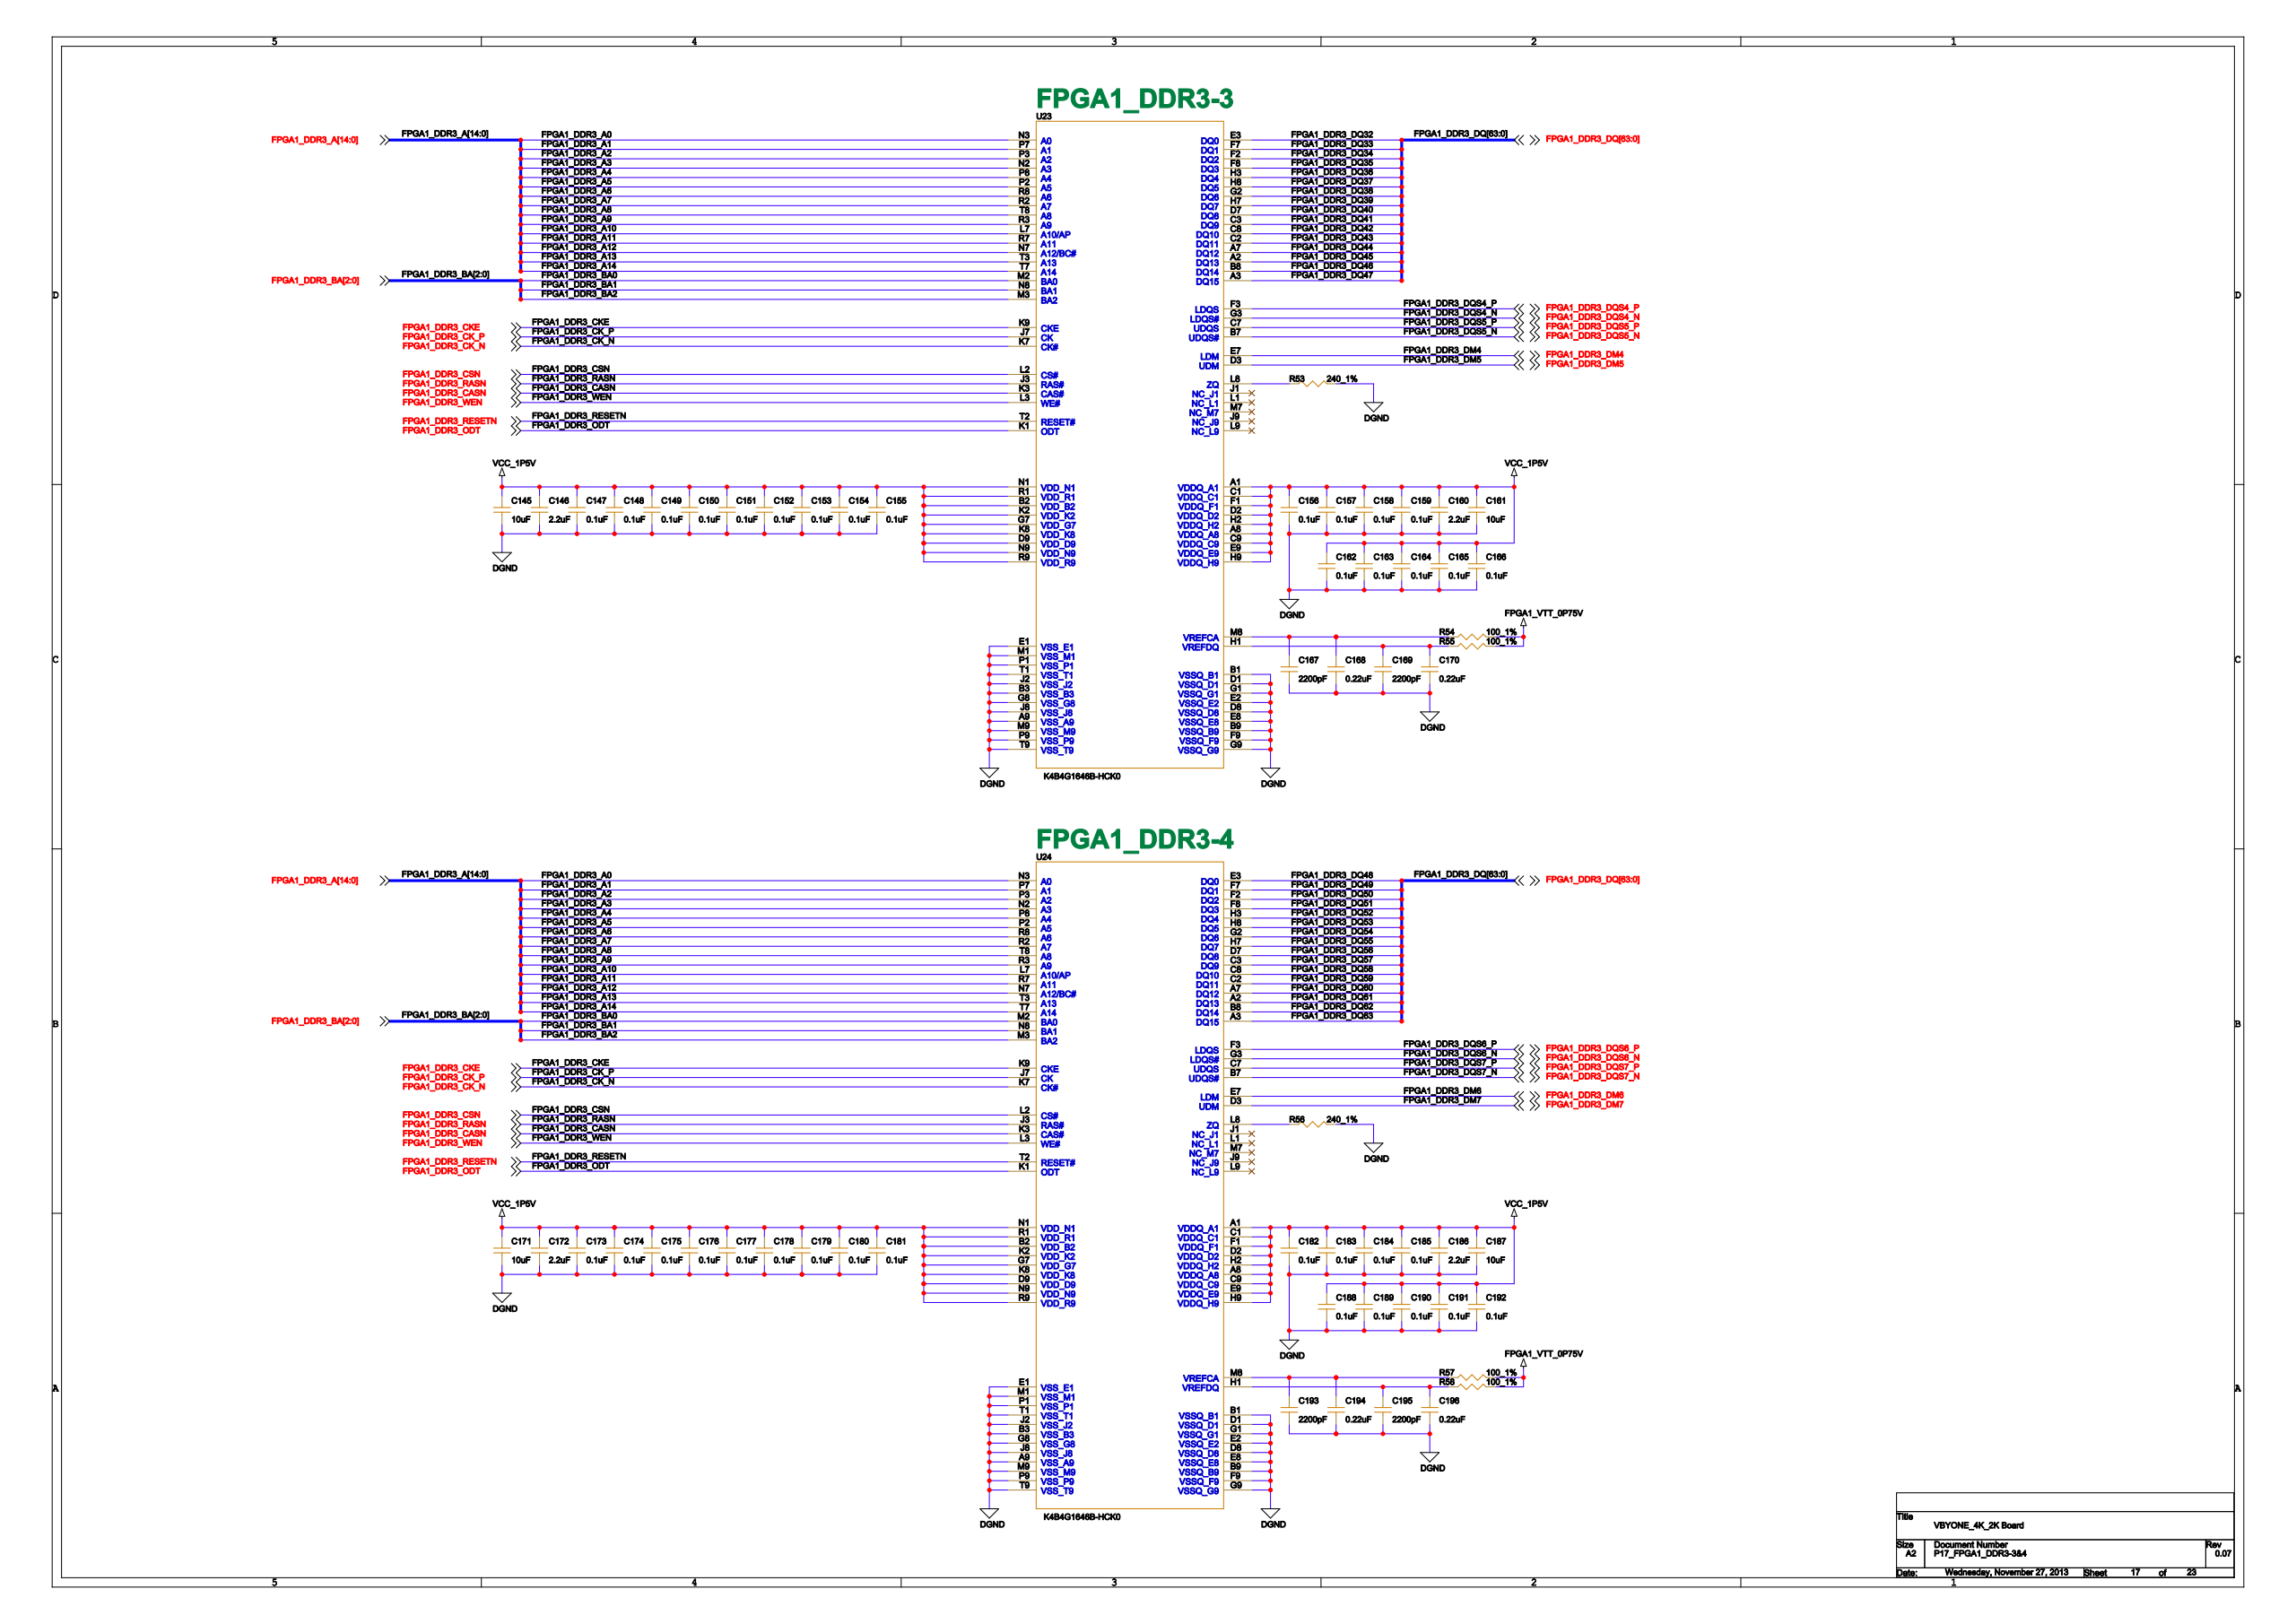Circuit board | Cadence Allegro | 1712 parts | 1495 nets | one sheet of the schematic
Parts on this sheet (reference | value | footprint):
C145 | 10uF | CRC2012RZAS
C146 | 2.2uF | CRC1608RZAS
C147 | 0.1uF | CRC1005RZAS
C148 | 0.1uF | CRC1005RZAS
C149 | 0.1uF | CRC1005RZAS
C150 | 0.1uF | CRC1005RZAS
C151 | 0.1uF | CRC1005RZAS
C152 | 0.1uF | CRC1005RZAS
C153 | 0.1uF | CRC1005RZAS
C154 | 0.1uF | CRC1005RZAS
C155 | 0.1uF | CRC1005RZAS
C156 | 0.1uF | CRC1005RZAS
C157 | 0.1uF | CRC1005RZAS
C158 | 0.1uF | CRC1005RZAS
C159 | 0.1uF | CRC1005RZAS
C160 | 2.2uF | CRC1608RZAS
C161 | 10uF | CRC2012RZAS
C162 | 0.1uF | CRC1005RZAS
C163 | 0.1uF | CRC1005RZAS
C164 | 0.1uF | CRC1005RZAS
C165 | 0.1uF | CRC1005RZAS
C166 | 0.1uF | CRC1005RZAS
C167 | 2200pF | CRC1608RZAS
C168 | 0.22uF | CRC1608RZAS
C169 | 2200pF | CRC1608RZAS
C170 | 0.22uF | CRC1608RZAS
C171 | 10uF | CRC2012RZAS
C172 | 2.2uF | CRC1608RZAS
C173 | 0.1uF | CRC1005RZAS
C174 | 0.1uF | CRC1005RZAS
C175 | 0.1uF | CRC1005RZAS
C176 | 0.1uF | CRC1005RZAS
C177 | 0.1uF | CRC1005RZAS
C178 | 0.1uF | CRC1005RZAS
C179 | 0.1uF | CRC1005RZAS
C180 | 0.1uF | CRC1005RZAS
C181 | 0.1uF | CRC1005RZAS
C182 | 0.1uF | CRC1005RZAS
C183 | 0.1uF | CRC1005RZAS
C184 | 0.1uF | CRC1005RZAS
C185 | 0.1uF | CRC1005RZAS
C186 | 2.2uF | CRC1608RZAS
C187 | 10uF | CRC2012RZAS
C188 | 0.1uF | CRC1005RZAS
C189 | 0.1uF | CRC1005RZAS
C190 | 0.1uF | CRC1005RZAS
C191 | 0.1uF | CRC1005RZAS
C192 | 0.1uF | CRC1005RZAS
C193 | 2200pF | CRC1608RZAS
C194 | 0.22uF | CRC1608RZAS
C195 | 2200pF | CRC1608RZAS
C196 | 0.22uF | CRC1608RZAS
R53 | 240_1% | CRC1608RZAS
R54 | 100_1% | CRC1005RZAS
R55 | 100_1% | CRC1005RZAS
R56 | 240_1% | CRC1608RZAS
R57 | 100_1% | CRC1005RZAS
R58 | 100_1% | CRC1005RZAS
U23 | K4B4G1646B-HCK0 | BGA096RFDS
U24 | K4B4G1646B-HCK0 | BGA096RFDS
Nets of these parts (net: part-pin ...):
DGND: C145-2 C146-2 C147-2 C148-2 C149-2 C150-2 C151-2 C152-2 C153-2 C154-2 C155-2 C156-2 C157-2 C158-2 C159-2 C160-2 C161-2 C162-2 C163-2 C164-2 C165-2 C166-2 C167-2 C168-2 C169-2 C170-2 C171-2 C172-2 C173-2 C174-2 C175-2 C176-2 C177-2 C178-2 C179-2 C180-2 C181-2 C182-2 C183-2 C184-2 C185-2 C186-2 C187-2 C188-2 C189-2 C190-2 C191-2 C192-2 C193-2 C194-2 C195-2 C196-2 R53-2 R56-2 U23-A9 U23-B1 U23-B3 U23-B9 U23-D1 U23-D8 U23-E1 U23-E2 U23-E8 U23-F9 U23-G1 U23-G8 U23-G9 U23-J2 U23-J8 U23-M1 U23-M9 U23-P1 U23-P9 U23-T1 U23-T9 U24-A9 U24-B1 U24-B3 U24-B9 U24-D1 U24-D8 U24-E1 U24-E2 U24-E8 U24-F9 U24-G1 U24-G8 U24-G9 U24-J2 U24-J8 U24-M1 U24-M9 U24-P1 U24-P9 U24-T1 U24-T9
VCC_1P5V: C145-1 C146-1 C147-1 C148-1 C149-1 C150-1 C151-1 C152-1 C153-1 C154-1 C155-1 C156-1 C157-1 C158-1 C159-1 C160-1 C161-1 C162-1 C163-1 C164-1 C165-1 C166-1 C171-1 C172-1 C173-1 C174-1 C175-1 C176-1 C177-1 C178-1 C179-1 C180-1 C181-1 C182-1 C183-1 C184-1 C185-1 C186-1 C187-1 C188-1 C189-1 C190-1 C191-1 C192-1 U23-A1 U23-A8 U23-B2 U23-C1 U23-C9 U23-D2 U23-D9 U23-E9 U23-F1 U23-G7 U23-H2 U23-H9 U23-K2 U23-K8 U23-N1 U23-N9 U23-R1 U23-R9 U24-A1 U24-A8 U24-B2 U24-C1 U24-C9 U24-D2 U24-D9 U24-E9 U24-F1 U24-G7 U24-H2 U24-H9 U24-K2 U24-K8 U24-N1 U24-N9 U24-R1 U24-R9
FPGA1_VTT_0P75V: R54-2 R55-2 R57-2 R58-2
N15095816: C167-1 C168-1 R54-1 U23-M8
N15095808: C169-1 C170-1 R55-1 U23-H1
N15101253: C193-1 C194-1 R57-1 U24-M8
N15101283: C195-1 C196-1 R58-1 U24-H1
FPGA1_DDR3_CKE: U23-K9 U24-K9
FPGA1_DDR3_RESETN: U23-T2 U24-T2
FPGA1_DDR3_ODT: U23-K1 U24-K1
FPGA1_DDR3_CSN: U23-L2 U24-L2
FPGA1_DDR3_A0: U23-N3 U24-N3
FPGA1_DDR3_A1: U23-P7 U24-P7
FPGA1_DDR3_A2: U23-P3 U24-P3
FPGA1_DDR3_A3: U23-N2 U24-N2
FPGA1_DDR3_A4: U23-P8 U24-P8
FPGA1_DDR3_A5: U23-P2 U24-P2
FPGA1_DDR3_A6: U23-R8 U24-R8
FPGA1_DDR3_A7: U23-R2 U24-R2
FPGA1_DDR3_A8: U23-T8 U24-T8
FPGA1_DDR3_A9: U23-R3 U24-R3
FPGA1_DDR3_A10: U23-L7 U24-L7
FPGA1_DDR3_A11: U23-R7 U24-R7
FPGA1_DDR3_A12: U23-N7 U24-N7
FPGA1_DDR3_A13: U23-T3 U24-T3
FPGA1_DDR3_BA0: U23-M2 U24-M2
FPGA1_DDR3_BA1: U23-N8 U24-N8
FPGA1_DDR3_BA2: U23-M3 U24-M3
FPGA1_DDR3_A14: U23-T7 U24-T7
FPGA1_DDR3_RASN: U23-J3 U24-J3
FPGA1_DDR3_CASN: U23-K3 U24-K3
FPGA1_DDR3_WEN: U23-L3 U24-L3
FPGA1_DDR3_CK_P: U23-J7 U24-J7
FPGA1_DDR3_CK_N: U23-K7 U24-K7
N15097740: R53-1 U23-L8
N15102855: R56-1 U24-L8
FPGA1_DDR3_DQ36: U23-H3
FPGA1_DDR3_DQ59: U24-C2
FPGA1_DDR3_DQ58: U24-C8
FPGA1_DDR3_DQ32: U23-E3
FPGA1_DDR3_DQ34: U23-F2
FPGA1_DDR3_DQ33: U23-F7
FPGA1_DDR3_DQ35: U23-F8
FPGA1_DDR3_DM7: U24-D3
FPGA1_DDR3_DQS7_N: U24-B7
FPGA1_DDR3_DQ57: U24-C3
FPGA1_DDR3_DQ56: U24-D7
FPGA1_DDR3_DQ63: U24-A3
FPGA1_DDR3_DM4: U23-E7
FPGA1_DDR3_DQS4_N: U23-G3
FPGA1_DDR3_DQS4_P: U23-F3
FPGA1_DDR3_DQ39: U23-H7
FPGA1_DDR3_DQ50: U24-F2
FPGA1_DDR3_DQS7_P: U24-C7
FPGA1_DDR3_DQ61: U24-A2
FPGA1_DDR3_DQ62: U24-B8
FPGA1_DDR3_DQ38: U23-G2
FPGA1_DDR3_DQ37: U23-H8
FPGA1_DDR3_DQ47: U23-A3
FPGA1_DDR3_DQ49: U24-F7
FPGA1_DDR3_DQ55: U24-H7
FPGA1_DDR3_DQ60: U24-A7
FPGA1_DDR3_DQS5_N: U23-B7
FPGA1_DDR3_DQS5_P: U23-C7
FPGA1_DDR3_DQ46: U23-B8
FPGA1_DDR3_DQ45: U23-A2
FPGA1_DDR3_DQ48: U24-E3
FPGA1_DDR3_DM6: U24-E7
FPGA1_DDR3_DQ52: U24-H3
FPGA1_DDR3_DQ51: U24-F8
FPGA1_DDR3_DQS6_N: U24-G3
FPGA1_DDR3_DQ40: U23-D7
FPGA1_DDR3_DM5: U23-D3
FPGA1_DDR3_DQ42: U23-C8
FPGA1_DDR3_DQ41: U23-C3
FPGA1_DDR3_DQ44: U23-A7
FPGA1_DDR3_DQ43: U23-C2
FPGA1_DDR3_DQ54: U24-G2
FPGA1_DDR3_DQ53: U24-H8
FPGA1_DDR3_DQS6_P: U24-F3